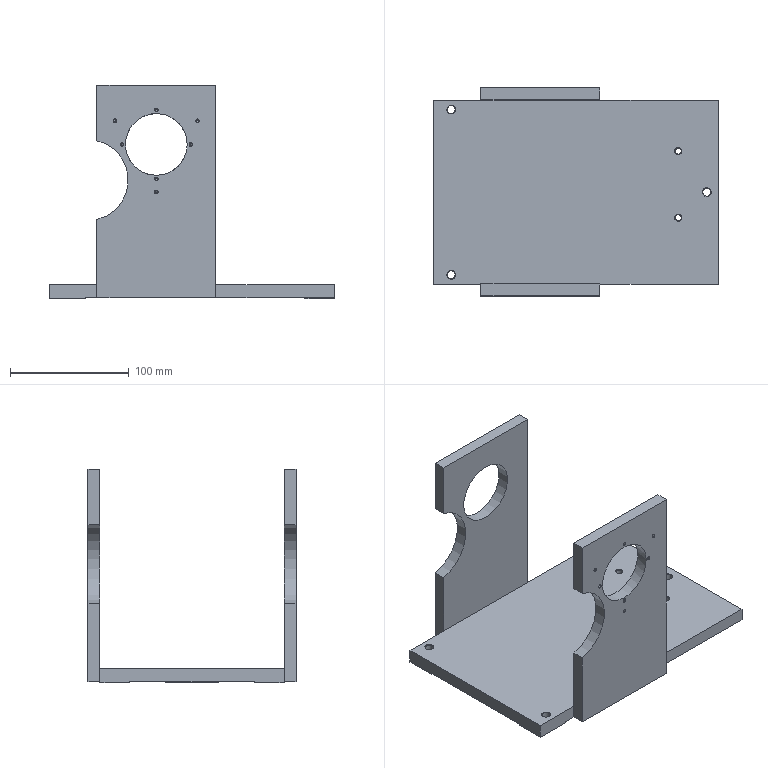Part | NX | features SIMPLE HOLE 18, SYMBOLIC_THREAD 15, DATUM_CSYS 12, SKETCH 11, HOLE PACKAGE 6, EXTRUDE 5 | 1 solid | 88 faces | box 240 x 175 x 180 mm | volume 699154 mm3 | cone 36 | plane 30 | cylinder 22 | commonest cylinder face diameters 2.5 x13 6.6 x3 5 x2 52 x2 68 x2